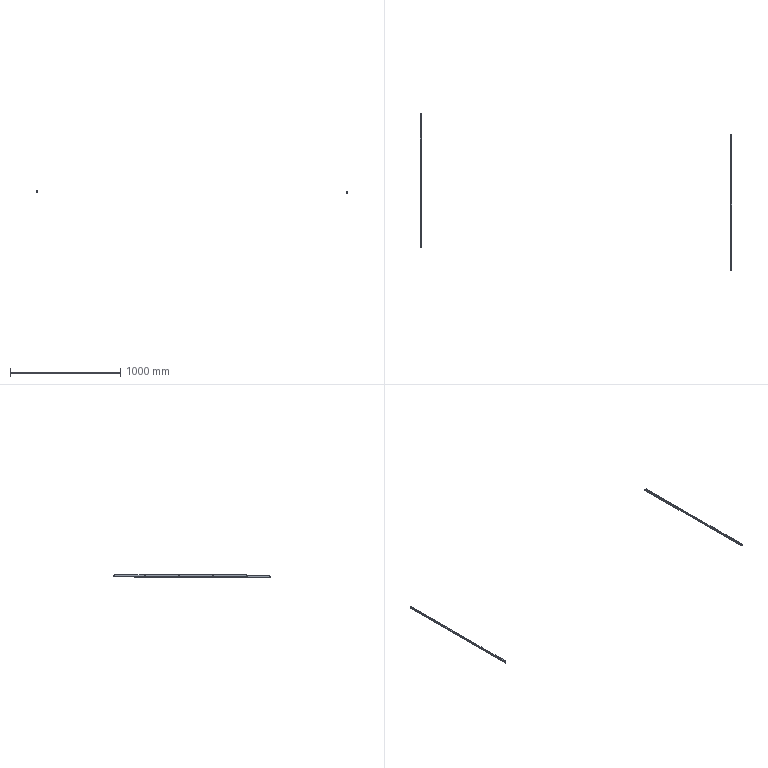NC program | NX | posted with a generic post | part box 2829 x 1430 x 20 mm
Whole program:
N10 G17 G21 G94 G90
(PLANAR_MILL_COPY_1 , TOOL : D16-48-D16-100-3T-FINISH)
N12 T01 M6
N14 G54
N16 G17 G0 G90 X623.5 Y0. S4000 M3
N18 G43 Z30. H1
N20 Z2.
N22 G94 G1 Z0. F1000.
N24 X610.5
N26 X-610.5
N28 X-623.5
N30 Z2.
N32 G0 Z30.
N34 M5
(动态粗_COPY , TOOL : D8-25-D8-60-3T-ROUGH)
N36 T02 M6
N38 G54
N40 G17 G0 G90 X-612.099 Y14.041 S6500 M3
N42 G43 Z30.2 H2
N44 Z-16.5
N46 G94 G1 X-612.096 Y14.017 Z-16.656 F3000.
N48 X-612.094 Y13.992 Z-16.718
N50 X-612.092 Y13.967 Z-16.763
N52 X-612.09 Y13.942 Z-16.8
N54 X-612.088 Y13.917 Z-16.831
N56 X-612.086 Y13.892 Z-16.857
N58 X-612.084 Y13.867 Z-16.88
N60 X-612.082 Y13.842 Z-16.9
N62 X-612.079 Y13.817 Z-16.918
N64 X-612.077 Y13.792 Z-16.933
N66 X-612.075 Y13.767 Z-16.947
N68 X-612.073 Y13.743 Z-16.958
N70 X-612.071 Y13.718 Z-16.968
N72 X-612.069 Y13.693 Z-16.977
N74 X-612.067 Y13.668 Z-16.984
N76 X-612.065 Y13.643 Z-16.99
N78 X-612.063 Y13.618 Z-16.994
N80 X-612.06 Y13.593 Z-16.997
N82 X-612.058 Y13.568 Z-16.999
N84 X-612.056 Y13.543 Z-17.
N86 X-611.941 Y12.189
N88 G3 X-611.521 Y11.547 R0.809
N90 X-608.852 Y10.809 R7.24
N92 X-602.467 Y10.524 R61.708
N94 G1 X-591.996 Y10.499
N96 X611.529 Y10.498
N98 G2 X614.518 Y8.975 R4.219
N100 X616.314 Y5.226 R8.476
N102 X616.908 Y-0.283 R28.763
N104 X616.964 Y-5.307 R81.71
N106 X615.222 Y-8.194 R4.462
N108 X611.247 Y-9.91 R9.208
N110 X605.653 Y-10.423 R33.747
N112 X592.304 Y-10.498 R644.658
N114 G1 X-611.522
N116 G2 X-614.51 Y-8.974 R4.211
N118 X-616.328 Y-5.15 R8.582
N120 X-616.905 Y0.21 R28.891
N122 X-616.966 Y5.309 R106.727
N124 X-614.44 Y8.626 R4.341
N126 X-610.74 Y9.498 R9.966
N128 X-608.267 Y9.577 R60.937
N130 G1 X606.21 Y9.57
N132 G2 X609.458 Y9.481 R56.895
N134 X610.737 Y9.173 R7.57
N136 G1 X611.435 Y9.095
N138 X612.322 Y8.784
N140 X613.119 Y8.284
N142 X613.784 Y7.619
N144 G2 X614.893 Y5.21 R7.513
N146 X615.807 Y-0.631 R25.525
N148 X615.843 Y-3.027 R15.649
N150 X614.645 Y-5.819 R5.747
N152 G1 X614.284 Y-6.822
N154 X613.784 Y-7.619
N156 X613.119 Y-8.284
N158 X612.322 Y-8.784
N160 X611.435 Y-9.095
N162 G2 X608.957 Y-9.266 R25.328
N164 X595.911 Y-9.494 R262.443
N166 G1 X590.061 Y-9.498
N168 X-608.971 Y-9.495
N170 G2 X-610.643 Y-9.184 R6.286
N172 G1 X-611.435 Y-9.095
N174 X-612.322 Y-8.784
N176 X-613.119 Y-8.284
N178 X-613.784 Y-7.619
N180 G2 X-614.891 Y-5.209 R7.502
N182 X-615.807 Y0.631 R25.577
N184 X-615.855 Y2.878 R16.821
N186 X-614.726 Y5.452 R4.975
N188 G3 X-614.595 Y5.935 R1.254
N190 G1 X-614.284 Y6.822
N192 X-613.784 Y7.619
N194 X-613.119 Y8.284
N196 X-612.322 Y8.784
N198 X-611.435 Y9.095
N200 X-610.5 Y9.2
N202 X610.501
N204 X611.435 Y9.095
N206 X612.322 Y8.784
N208 X613.119 Y8.284
N210 X613.784 Y7.619
N212 X614.284 Y6.822
N214 X614.595 Y5.935
N216 X614.7 Y4.999
N218 Y1.324
N220 G2 X614.7 Y-1.373 R13.82
N222 G1 Y-5.001
N224 G2 X614.57 Y-6.005 R36.316
N226 G3 X614.7 Y-5.001 R36.316
N228 G1 Y1.327
N230 Y-5.001
N232 X614.595 Y-5.935
N234 X614.284 Y-6.822
N236 X613.784 Y-7.619
N238 X613.119 Y-8.284
N240 X612.322 Y-8.784
N242 X611.435 Y-9.095
N244 G2 X610.199 Y-9.2 R8.458
N246 G1 X-610.501
N248 X-611.435 Y-9.095
N250 X-612.322 Y-8.784
N252 X-613.119 Y-8.284
N254 X-613.784 Y-7.619
N256 X-614.284 Y-6.822
N258 X-614.595 Y-5.935
N260 X-614.7 Y-4.999
N262 G3 X-614.762 Y0.374 R112.648
N264 G1 X-614.7 Y1.108
N266 Y5.001
N268 X-614.616 Y5.746
N270 X-614.7 Y5.001
N272 Y-1.367
N274 G2 X-615.655 Y-2.162 R0.808
N276 G1 X-616.656 Y-1.976
N278 X-616.68 Y-1.972 Z-16.999
N280 X-616.705 Y-1.967 Z-16.997
N282 X-616.73 Y-1.963 Z-16.994
N284 X-616.754 Y-1.958 Z-16.99
N286 X-616.779 Y-1.954 Z-16.984
N288 X-616.803 Y-1.949 Z-16.977
N290 X-616.828 Y-1.945 Z-16.968
N292 X-616.852 Y-1.94 Z-16.958
N294 X-616.877 Y-1.935 Z-16.947
N296 X-616.902 Y-1.931 Z-16.933
N298 X-616.926 Y-1.926 Z-16.918
N300 X-616.951 Y-1.922 Z-16.9
N302 X-616.975 Y-1.917 Z-16.88
N304 X-617. Y-1.913 Z-16.857
N306 X-617.025 Y-1.908 Z-16.831
N308 X-617.049 Y-1.904 Z-16.8
N310 X-617.074 Y-1.899 Z-16.763
N312 X-617.098 Y-1.894 Z-16.718
N314 X-617.123 Y-1.89 Z-16.656
N316 X-617.147 Y-1.885 Z-16.5
N318 G0 Z30.2
N320 M5
(PLANAR_MILL_1_COPY_1 , TOOL : D8-25-D8-60-3T-FINISH)
N322 T03 M6
N324 G54
N326 G17 G0 G90 X-614.5 Y-11.928 S4500 M3
N328 G43 Z30. H3
N330 Z-15.
N332 G94 G1 Z-17. F1000.
N334 Y-4.995
N336 Y9.
N338 X614.5
N340 Y-9.
N342 X-610.495
N344 X-617.428
N346 Z-15.
N348 G0 Z30.
N350 M5
(PLANAR_MILL_1_COPY_COPY , TOOL : 倒角D6-90度)
N352 T04 M6
N354 G54
N356 G17 G0 G90 X-612. Y-9.243 S4500 M3
N358 G43 Z30. H4
N360 Z0.5
N362 G94 G1 Z-1.5 F1000.
N364 Y-4.997
N366 Y6.5
N368 X612.
N370 Y-6.5
N372 X-610.497
N374 X-614.743
N376 Z0.5
N378 G0 Z30.
N380 M5
N382 M2